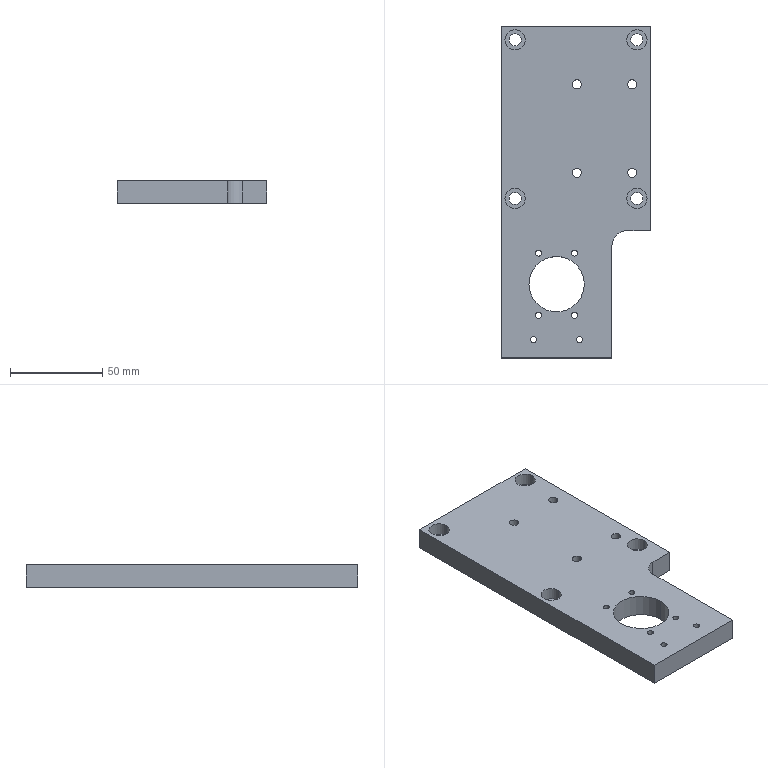Part | STEP file | X77-04016 | 1 solid | 51 faces | box 81 x 180 x 12 mm | volume 144400 mm3 | cylinder 39 | plane 12 | commonest cylinder face diameters 3.3 x12 5 x8 6.6 x8 11 x8 30 x2 16 x1